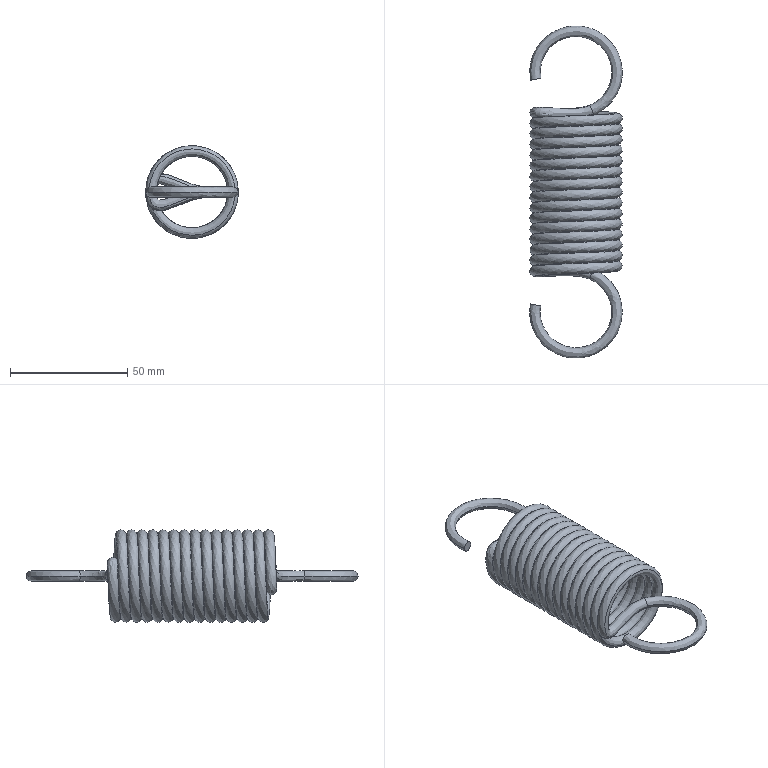Part | SolidWorks | features 3DProfileFeature 2, Helix 1, Sweep 1 | 1 solid | 8 faces | box 39.501 x 141.742 x 39.499 mm | volume 29526 mm3 | spline 6 | plane 2